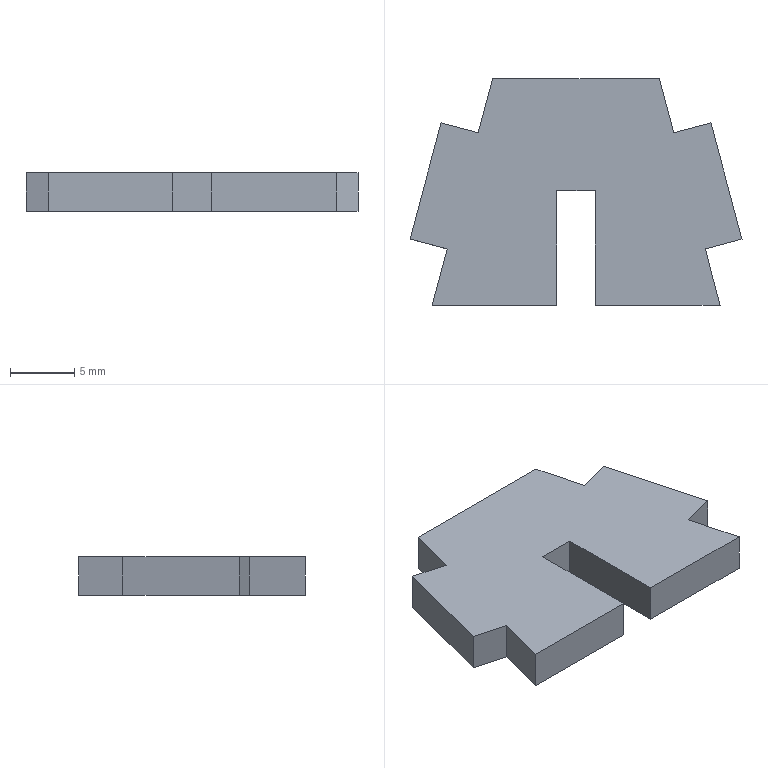Part | SolidWorks | features BaseBody 1 | 1 solid | 18 faces | box 25.93 x 17.686 x 3 mm | volume 1031 mm3 | plane 18
STEP:
#1=CARTESIAN_POINT('',(127.338,8.087,-1.5));
#2=VERTEX_POINT('',#1);
#3=CARTESIAN_POINT('',(127.338,-0.8444,-1.5));
#4=VERTEX_POINT('',#3);
#5=CARTESIAN_POINT('',(127.338,0.,-1.5));
#6=DIRECTION('',(0.,-1.,0.));
#7=VECTOR('',#6,1000.);
#8=LINE('',#5,#7);
#9=EDGE_CURVE('',#2,#4,#8,.T.);
#10=ORIENTED_EDGE('',*,*,#9,.T.);
#11=CARTESIAN_POINT('',(117.59,-0.8444,-1.5));
#12=VERTEX_POINT('',#11);
#13=CARTESIAN_POINT('',(0.,-0.8444,-1.5));
#14=DIRECTION('',(-1.,0.,0.));
#15=VECTOR('',#14,1000.);
#16=LINE('',#13,#15);
#17=EDGE_CURVE('',#4,#12,#16,.T.);
#18=ORIENTED_EDGE('',*,*,#17,.T.);
#19=CARTESIAN_POINT('',(118.767,3.542,-1.5));
#20=VERTEX_POINT('',#19);
#21=CARTESIAN_POINT('',(109.907,-29.485,-1.5));
#22=DIRECTION('',(0.2591,0.9658,0.));
#23=VECTOR('',#22,1000.);
#24=LINE('',#21,#23);
#25=EDGE_CURVE('',#12,#20,#24,.T.);
#26=ORIENTED_EDGE('',*,*,#25,.T.);
#27=CARTESIAN_POINT('',(115.871,4.318,-1.5));
#28=VERTEX_POINT('',#27);
#29=CARTESIAN_POINT('',(8.834,32.985,-1.5));
#30=DIRECTION('',(-0.966,0.2587,0.));
#31=VECTOR('',#30,1000.);
#32=LINE('',#29,#31);
#33=EDGE_CURVE('',#20,#28,#32,.T.);
#34=ORIENTED_EDGE('',*,*,#33,.T.);
#35=CARTESIAN_POINT('',(118.301,13.39,-1.5));
#36=VERTEX_POINT('',#35);
#37=CARTESIAN_POINT('',(107.037,-28.667,-1.5));
#38=DIRECTION('',(0.2587,0.966,0.));
#39=VECTOR('',#38,1000.);
#40=LINE('',#37,#39);
#41=EDGE_CURVE('',#28,#36,#40,.T.);
#42=ORIENTED_EDGE('',*,*,#41,.T.);
#43=CARTESIAN_POINT('',(121.196,12.614,-1.5));
#44=VERTEX_POINT('',#43);
#45=CARTESIAN_POINT('',(11.264,42.057,-1.5));
#46=DIRECTION('',(0.966,-0.2587,0.));
#47=VECTOR('',#46,1000.);
#48=LINE('',#45,#47);
#49=EDGE_CURVE('',#36,#44,#48,.T.);
#50=ORIENTED_EDGE('',*,*,#49,.T.);
#51=CARTESIAN_POINT('',(122.33,16.841,-1.5));
#52=VERTEX_POINT('',#51);
#53=CARTESIAN_POINT('',(109.917,-29.464,-1.5));
#54=DIRECTION('',(0.2589,0.9659,0.));
#55=VECTOR('',#54,1000.);
#56=LINE('',#53,#55);
#57=EDGE_CURVE('',#44,#52,#56,.T.);
#58=ORIENTED_EDGE('',*,*,#57,.T.);
#59=CARTESIAN_POINT('',(135.341,16.841,-1.5));
#60=VERTEX_POINT('',#59);
#61=CARTESIAN_POINT('',(0.,16.841,-1.5));
#62=DIRECTION('',(1.,0.,0.));
#63=VECTOR('',#62,1000.);
#64=LINE('',#61,#63);
#65=EDGE_CURVE('',#52,#60,#64,.T.);
#66=ORIENTED_EDGE('',*,*,#65,.T.);
#67=CARTESIAN_POINT('',(136.472,12.613,-1.5));
#68=VERTEX_POINT('',#67);
#69=CARTESIAN_POINT('',(130.506,34.912,-1.5));
#70=DIRECTION('',(0.2584,-0.966,0.));
#71=VECTOR('',#70,1000.);
#72=LINE('',#69,#71);
#73=EDGE_CURVE('',#60,#68,#72,.T.);
#74=ORIENTED_EDGE('',*,*,#73,.T.);
#75=CARTESIAN_POINT('',(139.371,13.39,-1.5));
#76=VERTEX_POINT('',#75);
#77=CARTESIAN_POINT('',(5.982,-22.335,-1.5));
#78=DIRECTION('',(0.966,0.2587,0.));
#79=VECTOR('',#78,1000.);
#80=LINE('',#77,#79);
#81=EDGE_CURVE('',#68,#76,#80,.T.);
#82=ORIENTED_EDGE('',*,*,#81,.T.);
#83=CARTESIAN_POINT('',(141.801,4.318,-1.5));
#84=VERTEX_POINT('',#83);
#85=CARTESIAN_POINT('',(133.389,35.725,-1.5));
#86=DIRECTION('',(0.2587,-0.966,0.));
#87=VECTOR('',#86,1000.);
#88=LINE('',#85,#87);
#89=EDGE_CURVE('',#76,#84,#88,.T.);
#90=ORIENTED_EDGE('',*,*,#89,.T.);
#91=CARTESIAN_POINT('',(138.932,3.55,-1.5));
#92=VERTEX_POINT('',#91);
#93=CARTESIAN_POINT('',(8.412,-31.407,-1.5));
#94=DIRECTION('',(-0.966,-0.2587,0.));
#95=VECTOR('',#94,1000.);
#96=LINE('',#93,#95);
#97=EDGE_CURVE('',#84,#92,#96,.T.);
#98=ORIENTED_EDGE('',*,*,#97,.T.);
#99=CARTESIAN_POINT('',(140.093,-0.8444,-1.5));
#100=VERTEX_POINT('',#99);
#101=CARTESIAN_POINT('',(130.739,34.55,-1.5));
#102=DIRECTION('',(0.2555,-0.9668,0.));
#103=VECTOR('',#102,1000.);
#104=LINE('',#101,#103);
#105=EDGE_CURVE('',#92,#100,#104,.T.);
#106=ORIENTED_EDGE('',*,*,#105,.T.);
#107=CARTESIAN_POINT('',(130.334,-0.8444,-1.5));
#108=VERTEX_POINT('',#107);
#109=CARTESIAN_POINT('',(0.,-0.8444,-1.5));
#110=DIRECTION('',(-1.,0.,0.));
#111=VECTOR('',#110,1000.);
#112=LINE('',#109,#111);
#113=EDGE_CURVE('',#100,#108,#112,.T.);
#114=ORIENTED_EDGE('',*,*,#113,.T.);
#115=CARTESIAN_POINT('',(130.334,8.087,-1.5));
#116=VERTEX_POINT('',#115);
#117=CARTESIAN_POINT('',(130.334,0.,-1.5));
#118=DIRECTION('',(0.,1.,0.));
#119=VECTOR('',#118,1000.);
#120=LINE('',#117,#119);
#121=EDGE_CURVE('',#108,#116,#120,.T.);
#122=ORIENTED_EDGE('',*,*,#121,.T.);
#123=CARTESIAN_POINT('',(0.,8.087,-1.5));
#124=DIRECTION('',(-1.,0.,0.));
#125=VECTOR('',#124,1000.);
#126=LINE('',#123,#125);
#127=EDGE_CURVE('',#116,#2,#126,.T.);
#128=ORIENTED_EDGE('',*,*,#127,.T.);
#129=EDGE_LOOP('',(#10,#18,#26,#34,#42,#50,#58,#66,#74,#82,#90,#98,#106,#114,#122,#128));
#130=FACE_OUTER_BOUND('',#129,.T.);
#131=CARTESIAN_POINT('',(0.,0.,-1.5));
#132=DIRECTION('',(0.,0.,1.));
#133=DIRECTION('',(1.,0.,0.));
#134=AXIS2_PLACEMENT_3D('',#131,#132,#133);
#135=PLANE('',#134);
#136=ADVANCED_FACE('',(#130),#135,.F.);
#137=CARTESIAN_POINT('',(127.338,8.087,1.5));
#138=VERTEX_POINT('',#137);
#139=CARTESIAN_POINT('',(127.338,-0.8444,1.5));
#140=VERTEX_POINT('',#139);
#141=CARTESIAN_POINT('',(127.338,0.,1.5));
#142=DIRECTION('',(0.,-1.,0.));
#143=VECTOR('',#142,1000.);
#144=LINE('',#141,#143);
#145=EDGE_CURVE('',#138,#140,#144,.T.);
#146=ORIENTED_EDGE('',*,*,#145,.F.);
#147=CARTESIAN_POINT('',(130.334,8.087,1.5));
#148=VERTEX_POINT('',#147);
#149=CARTESIAN_POINT('',(0.,8.087,1.5));
#150=DIRECTION('',(-1.,0.,0.));
#151=VECTOR('',#150,1000.);
#152=LINE('',#149,#151);
#153=EDGE_CURVE('',#148,#138,#152,.T.);
#154=ORIENTED_EDGE('',*,*,#153,.F.);
#155=CARTESIAN_POINT('',(130.334,-0.8444,1.5));
#156=VERTEX_POINT('',#155);
#157=CARTESIAN_POINT('',(130.334,0.,1.5));
#158=DIRECTION('',(0.,1.,0.));
#159=VECTOR('',#158,1000.);
#160=LINE('',#157,#159);
#161=EDGE_CURVE('',#156,#148,#160,.T.);
#162=ORIENTED_EDGE('',*,*,#161,.F.);
#163=CARTESIAN_POINT('',(140.093,-0.8444,1.5));
#164=VERTEX_POINT('',#163);
#165=CARTESIAN_POINT('',(0.,-0.8444,1.5));
#166=DIRECTION('',(-1.,0.,0.));
#167=VECTOR('',#166,1000.);
#168=LINE('',#165,#167);
#169=EDGE_CURVE('',#164,#156,#168,.T.);
#170=ORIENTED_EDGE('',*,*,#169,.F.);
#171=CARTESIAN_POINT('',(138.932,3.55,1.5));
#172=VERTEX_POINT('',#171);
#173=CARTESIAN_POINT('',(130.739,34.55,1.5));
#174=DIRECTION('',(0.2555,-0.9668,0.));
#175=VECTOR('',#174,1000.);
#176=LINE('',#173,#175);
#177=EDGE_CURVE('',#172,#164,#176,.T.);
#178=ORIENTED_EDGE('',*,*,#177,.F.);
#179=CARTESIAN_POINT('',(141.801,4.318,1.5));
#180=VERTEX_POINT('',#179);
#181=CARTESIAN_POINT('',(8.412,-31.407,1.5));
#182=DIRECTION('',(-0.966,-0.2587,0.));
#183=VECTOR('',#182,1000.);
#184=LINE('',#181,#183);
#185=EDGE_CURVE('',#180,#172,#184,.T.);
#186=ORIENTED_EDGE('',*,*,#185,.F.);
#187=CARTESIAN_POINT('',(139.371,13.39,1.5));
#188=VERTEX_POINT('',#187);
#189=CARTESIAN_POINT('',(133.389,35.725,1.5));
#190=DIRECTION('',(0.2587,-0.966,0.));
#191=VECTOR('',#190,1000.);
#192=LINE('',#189,#191);
#193=EDGE_CURVE('',#188,#180,#192,.T.);
#194=ORIENTED_EDGE('',*,*,#193,.F.);
#195=CARTESIAN_POINT('',(136.472,12.613,1.5));
#196=VERTEX_POINT('',#195);
#197=CARTESIAN_POINT('',(5.982,-22.335,1.5));
#198=DIRECTION('',(0.966,0.2587,0.));
#199=VECTOR('',#198,1000.);
#200=LINE('',#197,#199);
#201=EDGE_CURVE('',#196,#188,#200,.T.);
#202=ORIENTED_EDGE('',*,*,#201,.F.);
#203=CARTESIAN_POINT('',(135.341,16.841,1.5));
#204=VERTEX_POINT('',#203);
#205=CARTESIAN_POINT('',(130.506,34.912,1.5));
#206=DIRECTION('',(0.2584,-0.966,0.));
#207=VECTOR('',#206,1000.);
#208=LINE('',#205,#207);
#209=EDGE_CURVE('',#204,#196,#208,.T.);
#210=ORIENTED_EDGE('',*,*,#209,.F.);
#211=CARTESIAN_POINT('',(122.33,16.841,1.5));
#212=VERTEX_POINT('',#211);
#213=CARTESIAN_POINT('',(0.,16.841,1.5));
#214=DIRECTION('',(1.,0.,0.));
#215=VECTOR('',#214,1000.);
#216=LINE('',#213,#215);
#217=EDGE_CURVE('',#212,#204,#216,.T.);
#218=ORIENTED_EDGE('',*,*,#217,.F.);
#219=CARTESIAN_POINT('',(121.196,12.614,1.5));
#220=VERTEX_POINT('',#219);
#221=CARTESIAN_POINT('',(109.917,-29.464,1.5));
#222=DIRECTION('',(0.2589,0.9659,0.));
#223=VECTOR('',#222,1000.);
#224=LINE('',#221,#223);
#225=EDGE_CURVE('',#220,#212,#224,.T.);
#226=ORIENTED_EDGE('',*,*,#225,.F.);
#227=CARTESIAN_POINT('',(118.301,13.39,1.5));
#228=VERTEX_POINT('',#227);
#229=CARTESIAN_POINT('',(11.264,42.057,1.5));
#230=DIRECTION('',(0.966,-0.2587,0.));
#231=VECTOR('',#230,1000.);
#232=LINE('',#229,#231);
#233=EDGE_CURVE('',#228,#220,#232,.T.);
#234=ORIENTED_EDGE('',*,*,#233,.F.);
#235=CARTESIAN_POINT('',(115.871,4.318,1.5));
#236=VERTEX_POINT('',#235);
#237=CARTESIAN_POINT('',(107.037,-28.667,1.5));
#238=DIRECTION('',(0.2587,0.966,0.));
#239=VECTOR('',#238,1000.);
#240=LINE('',#237,#239);
#241=EDGE_CURVE('',#236,#228,#240,.T.);
#242=ORIENTED_EDGE('',*,*,#241,.F.);
#243=CARTESIAN_POINT('',(118.767,3.542,1.5));
#244=VERTEX_POINT('',#243);
#245=CARTESIAN_POINT('',(8.834,32.985,1.5));
#246=DIRECTION('',(-0.966,0.2587,0.));
#247=VECTOR('',#246,1000.);
#248=LINE('',#245,#247);
#249=EDGE_CURVE('',#244,#236,#248,.T.);
#250=ORIENTED_EDGE('',*,*,#249,.F.);
#251=CARTESIAN_POINT('',(117.59,-0.8444,1.5));
#252=VERTEX_POINT('',#251);
#253=CARTESIAN_POINT('',(109.907,-29.485,1.5));
#254=DIRECTION('',(0.2591,0.9658,0.));
#255=VECTOR('',#254,1000.);
#256=LINE('',#253,#255);
#257=EDGE_CURVE('',#252,#244,#256,.T.);
#258=ORIENTED_EDGE('',*,*,#257,.F.);
#259=CARTESIAN_POINT('',(0.,-0.8444,1.5));
#260=DIRECTION('',(-1.,0.,0.));
#261=VECTOR('',#260,1000.);
#262=LINE('',#259,#261);
#263=EDGE_CURVE('',#140,#252,#262,.T.);
#264=ORIENTED_EDGE('',*,*,#263,.F.);
#265=EDGE_LOOP('',(#146,#154,#162,#170,#178,#186,#194,#202,#210,#218,#226,#234,#242,#250,#258,#264));
#266=FACE_OUTER_BOUND('',#265,.T.);
#267=CARTESIAN_POINT('',(0.,0.,1.5));
#268=DIRECTION('',(0.,0.,1.));
#269=DIRECTION('',(1.,0.,0.));
#270=AXIS2_PLACEMENT_3D('',#267,#268,#269);
#271=PLANE('',#270);
#272=ADVANCED_FACE('',(#266),#271,.T.);
#273=ORIENTED_EDGE('',*,*,#17,.F.);
#274=CARTESIAN_POINT('',(127.338,-0.8444,1.5));
#275=DIRECTION('',(0.,0.,-1.));
#276=VECTOR('',#275,1000.);
#277=LINE('',#274,#276);
#278=EDGE_CURVE('',#140,#4,#277,.T.);
#279=ORIENTED_EDGE('',*,*,#278,.F.);
#280=ORIENTED_EDGE('',*,*,#263,.T.);
#281=CARTESIAN_POINT('',(117.59,-0.8444,1.5));
#282=DIRECTION('',(0.,0.,-1.));
#283=VECTOR('',#282,1000.);
#284=LINE('',#281,#283);
#285=EDGE_CURVE('',#252,#12,#284,.T.);
#286=ORIENTED_EDGE('',*,*,#285,.T.);
#287=EDGE_LOOP('',(#273,#279,#280,#286));
#288=FACE_OUTER_BOUND('',#287,.T.);
#289=CARTESIAN_POINT('',(0.,-0.8444,1.5));
#290=DIRECTION('',(0.,-1.,0.));
#291=DIRECTION('',(0.,0.,-1.));
#292=AXIS2_PLACEMENT_3D('',#289,#290,#291);
#293=PLANE('',#292);
#294=ADVANCED_FACE('',(#288),#293,.T.);
#295=ORIENTED_EDGE('',*,*,#25,.F.);
#296=ORIENTED_EDGE('',*,*,#285,.F.);
#297=ORIENTED_EDGE('',*,*,#257,.T.);
#298=CARTESIAN_POINT('',(118.767,3.542,1.5));
#299=DIRECTION('',(0.,0.,-1.));
#300=VECTOR('',#299,1000.);
#301=LINE('',#298,#300);
#302=EDGE_CURVE('',#244,#20,#301,.T.);
#303=ORIENTED_EDGE('',*,*,#302,.T.);
#304=EDGE_LOOP('',(#295,#296,#297,#303));
#305=FACE_OUTER_BOUND('',#304,.T.);
#306=CARTESIAN_POINT('',(109.907,-29.485,1.5));
#307=DIRECTION('',(-0.9658,0.2591,0.));
#308=DIRECTION('',(0.,0.,1.));
#309=AXIS2_PLACEMENT_3D('',#306,#307,#308);
#310=PLANE('',#309);
#311=ADVANCED_FACE('',(#305),#310,.T.);
#312=ORIENTED_EDGE('',*,*,#33,.F.);
#313=ORIENTED_EDGE('',*,*,#302,.F.);
#314=ORIENTED_EDGE('',*,*,#249,.T.);
#315=CARTESIAN_POINT('',(115.871,4.318,1.5));
#316=DIRECTION('',(0.,0.,-1.));
#317=VECTOR('',#316,1000.);
#318=LINE('',#315,#317);
#319=EDGE_CURVE('',#236,#28,#318,.T.);
#320=ORIENTED_EDGE('',*,*,#319,.T.);
#321=EDGE_LOOP('',(#312,#313,#314,#320));
#322=FACE_OUTER_BOUND('',#321,.T.);
#323=CARTESIAN_POINT('',(8.834,32.985,1.5));
#324=DIRECTION('',(-0.2587,-0.966,0.));
#325=DIRECTION('',(-0.966,0.2587,0.));
#326=AXIS2_PLACEMENT_3D('',#323,#324,#325);
#327=PLANE('',#326);
#328=ADVANCED_FACE('',(#322),#327,.T.);
#329=ORIENTED_EDGE('',*,*,#41,.F.);
#330=ORIENTED_EDGE('',*,*,#319,.F.);
#331=ORIENTED_EDGE('',*,*,#241,.T.);
#332=CARTESIAN_POINT('',(118.301,13.39,1.5));
#333=DIRECTION('',(0.,0.,-1.));
#334=VECTOR('',#333,1000.);
#335=LINE('',#332,#334);
#336=EDGE_CURVE('',#228,#36,#335,.T.);
#337=ORIENTED_EDGE('',*,*,#336,.T.);
#338=EDGE_LOOP('',(#329,#330,#331,#337));
#339=FACE_OUTER_BOUND('',#338,.T.);
#340=CARTESIAN_POINT('',(107.037,-28.667,1.5));
#341=DIRECTION('',(-0.966,0.2587,0.));
#342=DIRECTION('',(0.,0.,1.));
#343=AXIS2_PLACEMENT_3D('',#340,#341,#342);
#344=PLANE('',#343);
#345=ADVANCED_FACE('',(#339),#344,.T.);
#346=ORIENTED_EDGE('',*,*,#49,.F.);
#347=ORIENTED_EDGE('',*,*,#336,.F.);
#348=ORIENTED_EDGE('',*,*,#233,.T.);
#349=CARTESIAN_POINT('',(121.196,12.614,1.5));
#350=DIRECTION('',(0.,0.,-1.));
#351=VECTOR('',#350,1000.);
#352=LINE('',#349,#351);
#353=EDGE_CURVE('',#220,#44,#352,.T.);
#354=ORIENTED_EDGE('',*,*,#353,.T.);
#355=EDGE_LOOP('',(#346,#347,#348,#354));
#356=FACE_OUTER_BOUND('',#355,.T.);
#357=CARTESIAN_POINT('',(11.264,42.057,1.5));
#358=DIRECTION('',(0.2587,0.966,0.));
#359=DIRECTION('',(0.,0.,-1.));
#360=AXIS2_PLACEMENT_3D('',#357,#358,#359);
#361=PLANE('',#360);
#362=ADVANCED_FACE('',(#356),#361,.T.);
#363=ORIENTED_EDGE('',*,*,#57,.F.);
#364=ORIENTED_EDGE('',*,*,#353,.F.);
#365=ORIENTED_EDGE('',*,*,#225,.T.);
#366=CARTESIAN_POINT('',(122.33,16.841,1.5));
#367=DIRECTION('',(0.,0.,-1.));
#368=VECTOR('',#367,1000.);
#369=LINE('',#366,#368);
#370=EDGE_CURVE('',#212,#52,#369,.T.);
#371=ORIENTED_EDGE('',*,*,#370,.T.);
#372=EDGE_LOOP('',(#363,#364,#365,#371));
#373=FACE_OUTER_BOUND('',#372,.T.);
#374=CARTESIAN_POINT('',(109.917,-29.464,1.5));
#375=DIRECTION('',(-0.9659,0.2589,0.));
#376=DIRECTION('',(0.,0.,1.));
#377=AXIS2_PLACEMENT_3D('',#374,#375,#376);
#378=PLANE('',#377);
#379=ADVANCED_FACE('',(#373),#378,.T.);
#380=ORIENTED_EDGE('',*,*,#65,.F.);
#381=ORIENTED_EDGE('',*,*,#370,.F.);
#382=ORIENTED_EDGE('',*,*,#217,.T.);
#383=CARTESIAN_POINT('',(135.341,16.841,1.5));
#384=DIRECTION('',(0.,0.,-1.));
#385=VECTOR('',#384,1000.);
#386=LINE('',#383,#385);
#387=EDGE_CURVE('',#204,#60,#386,.T.);
#388=ORIENTED_EDGE('',*,*,#387,.T.);
#389=EDGE_LOOP('',(#380,#381,#382,#388));
#390=FACE_OUTER_BOUND('',#389,.T.);
#391=CARTESIAN_POINT('',(0.,16.841,1.5));
#392=DIRECTION('',(0.,1.,0.));
#393=DIRECTION('',(1.,0.,0.));
#394=AXIS2_PLACEMENT_3D('',#391,#392,#393);
#395=PLANE('',#394);
#396=ADVANCED_FACE('',(#390),#395,.T.);
#397=ORIENTED_EDGE('',*,*,#73,.F.);
#398=ORIENTED_EDGE('',*,*,#387,.F.);
#399=ORIENTED_EDGE('',*,*,#209,.T.);
#400=CARTESIAN_POINT('',(136.472,12.613,1.5));
#401=DIRECTION('',(0.,0.,-1.));
#402=VECTOR('',#401,1000.);
#403=LINE('',#400,#402);
#404=EDGE_CURVE('',#196,#68,#403,.T.);
#405=ORIENTED_EDGE('',*,*,#404,.T.);
#406=EDGE_LOOP('',(#397,#398,#399,#405));
#407=FACE_OUTER_BOUND('',#406,.T.);
#408=CARTESIAN_POINT('',(130.506,34.912,1.5));
#409=DIRECTION('',(0.966,0.2584,0.));
#410=DIRECTION('',(0.,0.,-1.));
#411=AXIS2_PLACEMENT_3D('',#408,#409,#410);
#412=PLANE('',#411);
#413=ADVANCED_FACE('',(#407),#412,.T.);
#414=ORIENTED_EDGE('',*,*,#81,.F.);
#415=ORIENTED_EDGE('',*,*,#404,.F.);
#416=ORIENTED_EDGE('',*,*,#201,.T.);
#417=CARTESIAN_POINT('',(139.371,13.39,1.5));
#418=DIRECTION('',(0.,0.,-1.));
#419=VECTOR('',#418,1000.);
#420=LINE('',#417,#419);
#421=EDGE_CURVE('',#188,#76,#420,.T.);
#422=ORIENTED_EDGE('',*,*,#421,.T.);
#423=EDGE_LOOP('',(#414,#415,#416,#422));
#424=FACE_OUTER_BOUND('',#423,.T.);
#425=CARTESIAN_POINT('',(5.982,-22.335,1.5));
#426=DIRECTION('',(-0.2587,0.966,0.));
#427=DIRECTION('',(0.,0.,1.));
#428=AXIS2_PLACEMENT_3D('',#425,#426,#427);
#429=PLANE('',#428);
#430=ADVANCED_FACE('',(#424),#429,.T.);
#431=ORIENTED_EDGE('',*,*,#89,.F.);
#432=ORIENTED_EDGE('',*,*,#421,.F.);
#433=ORIENTED_EDGE('',*,*,#193,.T.);
#434=CARTESIAN_POINT('',(141.801,4.318,1.5));
#435=DIRECTION('',(0.,0.,-1.));
#436=VECTOR('',#435,1000.);
#437=LINE('',#434,#436);
#438=EDGE_CURVE('',#180,#84,#437,.T.);
#439=ORIENTED_EDGE('',*,*,#438,.T.);
#440=EDGE_LOOP('',(#431,#432,#433,#439));
#441=FACE_OUTER_BOUND('',#440,.T.);
#442=CARTESIAN_POINT('',(133.389,35.725,1.5));
#443=DIRECTION('',(0.966,0.2587,0.));
#444=DIRECTION('',(0.,0.,-1.));
#445=AXIS2_PLACEMENT_3D('',#442,#443,#444);
#446=PLANE('',#445);
#447=ADVANCED_FACE('',(#441),#446,.T.);
#448=ORIENTED_EDGE('',*,*,#97,.F.);
#449=ORIENTED_EDGE('',*,*,#438,.F.);
#450=ORIENTED_EDGE('',*,*,#185,.T.);
#451=CARTESIAN_POINT('',(138.932,3.55,1.5));
#452=DIRECTION('',(0.,0.,-1.));
#453=VECTOR('',#452,1000.);
#454=LINE('',#451,#453);
#455=EDGE_CURVE('',#172,#92,#454,.T.);
#456=ORIENTED_EDGE('',*,*,#455,.T.);
#457=EDGE_LOOP('',(#448,#449,#450,#456));
#458=FACE_OUTER_BOUND('',#457,.T.);
#459=CARTESIAN_POINT('',(8.412,-31.407,1.5));
#460=DIRECTION('',(0.2587,-0.966,0.));
#461=DIRECTION('',(0.,0.,-1.));
#462=AXIS2_PLACEMENT_3D('',#459,#460,#461);
#463=PLANE('',#462);
#464=ADVANCED_FACE('',(#458),#463,.T.);
#465=ORIENTED_EDGE('',*,*,#105,.F.);
#466=ORIENTED_EDGE('',*,*,#455,.F.);
#467=ORIENTED_EDGE('',*,*,#177,.T.);
#468=CARTESIAN_POINT('',(140.093,-0.8444,1.5));
#469=DIRECTION('',(0.,0.,-1.));
#470=VECTOR('',#469,1000.);
#471=LINE('',#468,#470);
#472=EDGE_CURVE('',#164,#100,#471,.T.);
#473=ORIENTED_EDGE('',*,*,#472,.T.);
#474=EDGE_LOOP('',(#465,#466,#467,#473));
#475=FACE_OUTER_BOUND('',#474,.T.);
#476=CARTESIAN_POINT('',(130.739,34.55,1.5));
#477=DIRECTION('',(0.9668,0.2555,0.));
#478=DIRECTION('',(0.,0.,-1.));
#479=AXIS2_PLACEMENT_3D('',#476,#477,#478);
#480=PLANE('',#479);
#481=ADVANCED_FACE('',(#475),#480,.T.);
#482=ORIENTED_EDGE('',*,*,#113,.F.);
#483=ORIENTED_EDGE('',*,*,#472,.F.);
#484=ORIENTED_EDGE('',*,*,#169,.T.);
#485=CARTESIAN_POINT('',(130.334,-0.8444,1.5));
#486=DIRECTION('',(0.,0.,-1.));
#487=VECTOR('',#486,1000.);
#488=LINE('',#485,#487);
#489=EDGE_CURVE('',#156,#108,#488,.T.);
#490=ORIENTED_EDGE('',*,*,#489,.T.);
#491=EDGE_LOOP('',(#482,#483,#484,#490));
#492=FACE_OUTER_BOUND('',#491,.T.);
#493=CARTESIAN_POINT('',(0.,-0.8444,1.5));
#494=DIRECTION('',(0.,-1.,0.));
#495=DIRECTION('',(0.,0.,-1.));
#496=AXIS2_PLACEMENT_3D('',#493,#494,#495);
#497=PLANE('',#496);
#498=ADVANCED_FACE('',(#492),#497,.T.);
#499=ORIENTED_EDGE('',*,*,#121,.F.);
#500=ORIENTED_EDGE('',*,*,#489,.F.);
#501=ORIENTED_EDGE('',*,*,#161,.T.);
#502=CARTESIAN_POINT('',(130.334,8.087,1.5));
#503=DIRECTION('',(0.,0.,-1.));
#504=VECTOR('',#503,1000.);
#505=LINE('',#502,#504);
#506=EDGE_CURVE('',#148,#116,#505,.T.);
#507=ORIENTED_EDGE('',*,*,#506,.T.);
#508=EDGE_LOOP('',(#499,#500,#501,#507));
#509=FACE_OUTER_BOUND('',#508,.T.);
#510=CARTESIAN_POINT('',(130.334,0.,1.5));
#511=DIRECTION('',(-1.,0.,0.));
#512=DIRECTION('',(0.,0.,1.));
#513=AXIS2_PLACEMENT_3D('',#510,#511,#512);
#514=PLANE('',#513);
#515=ADVANCED_FACE('',(#509),#514,.T.);
#516=ORIENTED_EDGE('',*,*,#127,.F.);
#517=ORIENTED_EDGE('',*,*,#506,.F.);
#518=ORIENTED_EDGE('',*,*,#153,.T.);
#519=CARTESIAN_POINT('',(127.338,8.087,1.5));
#520=DIRECTION('',(0.,0.,-1.));
#521=VECTOR('',#520,1000.);
#522=LINE('',#519,#521);
#523=EDGE_CURVE('',#138,#2,#522,.T.);
#524=ORIENTED_EDGE('',*,*,#523,.T.);
#525=EDGE_LOOP('',(#516,#517,#518,#524));
#526=FACE_OUTER_BOUND('',#525,.T.);
#527=CARTESIAN_POINT('',(0.,8.087,1.5));
#528=DIRECTION('',(0.,-1.,0.));
#529=DIRECTION('',(0.,0.,-1.));
#530=AXIS2_PLACEMENT_3D('',#527,#528,#529);
#531=PLANE('',#530);
#532=ADVANCED_FACE('',(#526),#531,.T.);
#533=ORIENTED_EDGE('',*,*,#9,.F.);
#534=ORIENTED_EDGE('',*,*,#523,.F.);
#535=ORIENTED_EDGE('',*,*,#145,.T.);
#536=ORIENTED_EDGE('',*,*,#278,.T.);
#537=EDGE_LOOP('',(#533,#534,#535,#536));
#538=FACE_OUTER_BOUND('',#537,.T.);
#539=CARTESIAN_POINT('',(127.338,0.,1.5));
#540=DIRECTION('',(1.,0.,0.));
#541=DIRECTION('',(0.,1.,0.));
#542=AXIS2_PLACEMENT_3D('',#539,#540,#541);
#543=PLANE('',#542);
#544=ADVANCED_FACE('',(#538),#543,.T.);
#545=CLOSED_SHELL('',(#136,#272,#294,#311,#328,#345,#362,#379,#396,#413,#430,#447,#464,#481,#498,#515,#532,#544));
#546=MANIFOLD_SOLID_BREP('',#545);
#547=CARTESIAN_POINT('',(0.,0.,0.));
#548=DIRECTION('',(0.,0.,1.));
#549=DIRECTION('',(1.,0.,0.));
#550=AXIS2_PLACEMENT_3D('',#547,#548,#549);
#551=(LENGTH_UNIT()NAMED_UNIT(*)SI_UNIT(.MILLI.,.METRE.));
#552=UNCERTAINTY_MEASURE_WITH_UNIT(LENGTH_MEASURE(0.00001),#551,'','');
#553=(NAMED_UNIT(*)PLANE_ANGLE_UNIT()SI_UNIT($,.RADIAN.));
#554=(NAMED_UNIT(*)SI_UNIT($,.STERADIAN.)SOLID_ANGLE_UNIT());
#555=(GEOMETRIC_REPRESENTATION_CONTEXT(3)GLOBAL_UNCERTAINTY_ASSIGNED_CONTEXT((#552))GLOBAL_UNIT_ASSIGNED_CONTEXT((#551,#553,#554))REPRESENTATION_CONTEXT('',''));
#556=ADVANCED_BREP_SHAPE_REPRESENTATION('',(#546,#550),#555);